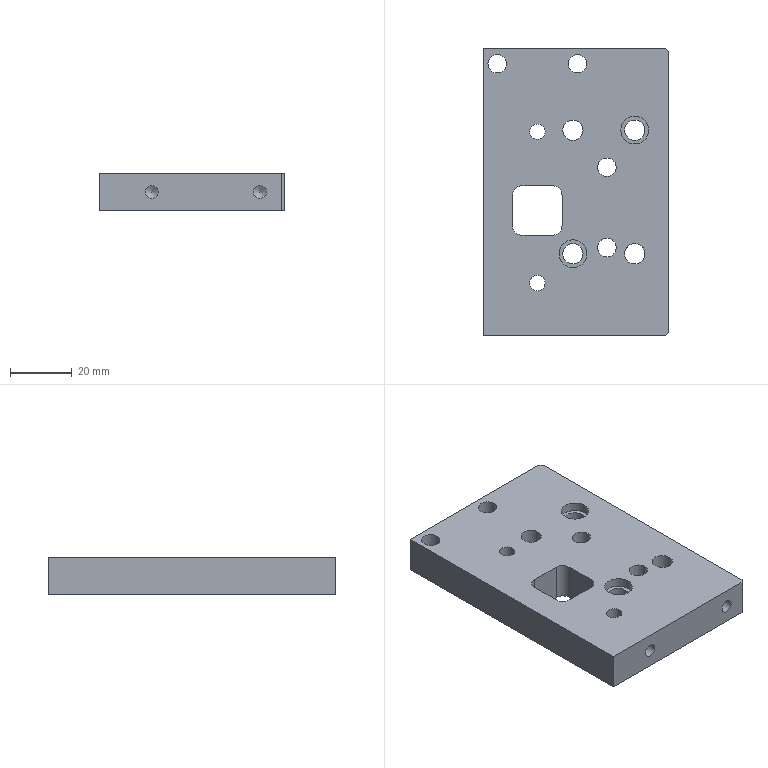Part | NX | features BREP 1 | 1 solid | 46 faces | box 60 x 93 x 12 mm | volume 58492 mm3 | cylinder 24 | plane 18 | cone 4 | commonest cylinder face diameters 6 x8 4.2 x4 6.6 x4 11 x4 5 x2 9 x2
STEP:
#1=CARTESIAN_POINT('',(29.,46.5,12.));
#2=VERTEX_POINT('',#1);
#3=CARTESIAN_POINT('',(-30.,46.5,12.));
#4=VERTEX_POINT('',#3);
#5=CARTESIAN_POINT('',(0.,46.5,12.));
#6=DIRECTION('',(-1.,0.,0.));
#7=VECTOR('',#6,1000.);
#8=LINE('',#5,#7);
#9=EDGE_CURVE('',#2,#4,#8,.T.);
#10=ORIENTED_EDGE('',*,*,#9,.T.);
#11=CARTESIAN_POINT('',(-30.,-46.5,12.));
#12=VERTEX_POINT('',#11);
#13=CARTESIAN_POINT('',(-30.,0.,12.));
#14=DIRECTION('',(0.,-1.,0.));
#15=VECTOR('',#14,1000.);
#16=LINE('',#13,#15);
#17=EDGE_CURVE('',#4,#12,#16,.T.);
#18=ORIENTED_EDGE('',*,*,#17,.T.);
#19=CARTESIAN_POINT('',(29.,-46.5,12.));
#20=VERTEX_POINT('',#19);
#21=CARTESIAN_POINT('',(0.,-46.5,12.));
#22=DIRECTION('',(1.,0.,0.));
#23=VECTOR('',#22,1000.);
#24=LINE('',#21,#23);
#25=EDGE_CURVE('',#12,#20,#24,.T.);
#26=ORIENTED_EDGE('',*,*,#25,.T.);
#27=CARTESIAN_POINT('',(30.,-45.5,12.));
#28=VERTEX_POINT('',#27);
#29=CARTESIAN_POINT('',(30.,-45.5,12.));
#30=DIRECTION('',(0.7071,0.7071,0.));
#31=VECTOR('',#30,1000.);
#32=LINE('',#29,#31);
#33=EDGE_CURVE('',#20,#28,#32,.T.);
#34=ORIENTED_EDGE('',*,*,#33,.T.);
#35=CARTESIAN_POINT('',(30.,45.5,12.));
#36=VERTEX_POINT('',#35);
#37=CARTESIAN_POINT('',(30.,0.,12.));
#38=DIRECTION('',(0.,1.,0.));
#39=VECTOR('',#38,1000.);
#40=LINE('',#37,#39);
#41=EDGE_CURVE('',#28,#36,#40,.T.);
#42=ORIENTED_EDGE('',*,*,#41,.T.);
#43=CARTESIAN_POINT('',(29.,46.5,12.));
#44=DIRECTION('',(-0.7071,0.7071,0.));
#45=VECTOR('',#44,1000.);
#46=LINE('',#43,#45);
#47=EDGE_CURVE('',#36,#2,#46,.T.);
#48=ORIENTED_EDGE('',*,*,#47,.T.);
#49=EDGE_LOOP('',(#10,#18,#26,#34,#42,#48));
#50=FACE_BOUND('',#49,.T.);
#51=CARTESIAN_POINT('',(-4.5,-1.,12.));
#52=VERTEX_POINT('',#51);
#53=CARTESIAN_POINT('',(-4.5,-11.,12.));
#54=VERTEX_POINT('',#53);
#55=CARTESIAN_POINT('',(-4.5,0.,12.));
#56=DIRECTION('',(0.,-1.,0.));
#57=VECTOR('',#56,1000.);
#58=LINE('',#55,#57);
#59=EDGE_CURVE('',#52,#54,#58,.T.);
#60=ORIENTED_EDGE('',*,*,#59,.T.);
#61=CARTESIAN_POINT('',(-7.5,-14.,12.));
#62=VERTEX_POINT('',#61);
#63=CARTESIAN_POINT('',(-7.5,-11.,12.));
#64=DIRECTION('',(0.,0.,-1.));
#65=DIRECTION('',(1.,0.,0.));
#66=AXIS2_PLACEMENT_3D('',#63,#64,#65);
#67=CIRCLE('',#66,3.);
#68=EDGE_CURVE('',#54,#62,#67,.T.);
#69=ORIENTED_EDGE('',*,*,#68,.T.);
#70=CARTESIAN_POINT('',(-17.5,-14.,12.));
#71=VERTEX_POINT('',#70);
#72=CARTESIAN_POINT('',(0.,-14.,12.));
#73=DIRECTION('',(-1.,0.,0.));
#74=VECTOR('',#73,1000.);
#75=LINE('',#72,#74);
#76=EDGE_CURVE('',#62,#71,#75,.T.);
#77=ORIENTED_EDGE('',*,*,#76,.T.);
#78=CARTESIAN_POINT('',(-20.5,-11.,12.));
#79=VERTEX_POINT('',#78);
#80=CARTESIAN_POINT('',(-17.5,-11.,12.));
#81=DIRECTION('',(0.,0.,-1.));
#82=DIRECTION('',(1.,0.,0.));
#83=AXIS2_PLACEMENT_3D('',#80,#81,#82);
#84=CIRCLE('',#83,3.);
#85=EDGE_CURVE('',#71,#79,#84,.T.);
#86=ORIENTED_EDGE('',*,*,#85,.T.);
#87=CARTESIAN_POINT('',(-20.5,-1.,12.));
#88=VERTEX_POINT('',#87);
#89=CARTESIAN_POINT('',(-20.5,0.,12.));
#90=DIRECTION('',(0.,1.,0.));
#91=VECTOR('',#90,1000.);
#92=LINE('',#89,#91);
#93=EDGE_CURVE('',#79,#88,#92,.T.);
#94=ORIENTED_EDGE('',*,*,#93,.T.);
#95=CARTESIAN_POINT('',(-17.5,2.,12.));
#96=VERTEX_POINT('',#95);
#97=CARTESIAN_POINT('',(-17.5,-1.,12.));
#98=DIRECTION('',(0.,0.,-1.));
#99=DIRECTION('',(1.,0.,0.));
#100=AXIS2_PLACEMENT_3D('',#97,#98,#99);
#101=CIRCLE('',#100,3.);
#102=EDGE_CURVE('',#88,#96,#101,.T.);
#103=ORIENTED_EDGE('',*,*,#102,.T.);
#104=CARTESIAN_POINT('',(-7.5,2.,12.));
#105=VERTEX_POINT('',#104);
#106=CARTESIAN_POINT('',(0.,2.,12.));
#107=DIRECTION('',(1.,0.,0.));
#108=VECTOR('',#107,1000.);
#109=LINE('',#106,#108);
#110=EDGE_CURVE('',#96,#105,#109,.T.);
#111=ORIENTED_EDGE('',*,*,#110,.T.);
#112=CARTESIAN_POINT('',(-7.5,-1.,12.));
#113=DIRECTION('',(0.,0.,-1.));
#114=DIRECTION('',(1.,0.,0.));
#115=AXIS2_PLACEMENT_3D('',#112,#113,#114);
#116=CIRCLE('',#115,3.);
#117=EDGE_CURVE('',#105,#52,#116,.T.);
#118=ORIENTED_EDGE('',*,*,#117,.T.);
#119=EDGE_LOOP('',(#60,#69,#77,#86,#94,#103,#111,#118));
#120=FACE_BOUND('',#119,.T.);
#121=CARTESIAN_POINT('',(-15.,-29.5,12.));
#122=VERTEX_POINT('',#121);
#123=CARTESIAN_POINT('',(-12.5,-29.5,12.));
#124=DIRECTION('',(0.,0.,-1.));
#125=DIRECTION('',(-1.,0.,0.));
#126=AXIS2_PLACEMENT_3D('',#123,#124,#125);
#127=CIRCLE('',#126,2.5);
#128=EDGE_CURVE('',#122,#122,#127,.T.);
#129=ORIENTED_EDGE('',*,*,#128,.T.);
#130=EDGE_LOOP('',(#129));
#131=FACE_BOUND('',#130,.T.);
#132=CARTESIAN_POINT('',(-15.,19.5,12.));
#133=VERTEX_POINT('',#132);
#134=CARTESIAN_POINT('',(-12.5,19.5,12.));
#135=DIRECTION('',(0.,0.,-1.));
#136=DIRECTION('',(-1.,0.,0.));
#137=AXIS2_PLACEMENT_3D('',#134,#135,#136);
#138=CIRCLE('',#137,2.5);
#139=EDGE_CURVE('',#133,#133,#138,.T.);
#140=ORIENTED_EDGE('',*,*,#139,.T.);
#141=EDGE_LOOP('',(#140));
#142=FACE_BOUND('',#141,.T.);
#143=CARTESIAN_POINT('',(15.7,-20.,12.));
#144=VERTEX_POINT('',#143);
#145=CARTESIAN_POINT('',(19.,-20.,12.));
#146=DIRECTION('',(0.,0.,-1.));
#147=DIRECTION('',(-1.,0.,0.));
#148=AXIS2_PLACEMENT_3D('',#145,#146,#147);
#149=CIRCLE('',#148,3.3);
#150=EDGE_CURVE('',#144,#144,#149,.T.);
#151=ORIENTED_EDGE('',*,*,#150,.T.);
#152=EDGE_LOOP('',(#151));
#153=FACE_BOUND('',#152,.T.);
#154=CARTESIAN_POINT('',(-4.3,20.,12.));
#155=VERTEX_POINT('',#154);
#156=CARTESIAN_POINT('',(-1.,20.,12.));
#157=DIRECTION('',(0.,0.,-1.));
#158=DIRECTION('',(-1.,0.,0.));
#159=AXIS2_PLACEMENT_3D('',#156,#157,#158);
#160=CIRCLE('',#159,3.3);
#161=EDGE_CURVE('',#155,#155,#160,.T.);
#162=ORIENTED_EDGE('',*,*,#161,.T.);
#163=EDGE_LOOP('',(#162));
#164=FACE_BOUND('',#163,.T.);
#165=CARTESIAN_POINT('',(7.,8.,12.));
#166=VERTEX_POINT('',#165);
#167=CARTESIAN_POINT('',(10.,8.,12.));
#168=DIRECTION('',(0.,0.,-1.));
#169=DIRECTION('',(-1.,0.,0.));
#170=AXIS2_PLACEMENT_3D('',#167,#168,#169);
#171=CIRCLE('',#170,3.);
#172=EDGE_CURVE('',#166,#166,#171,.T.);
#173=ORIENTED_EDGE('',*,*,#172,.T.);
#174=EDGE_LOOP('',(#173));
#175=FACE_BOUND('',#174,.T.);
#176=CARTESIAN_POINT('',(7.,-18.,12.));
#177=VERTEX_POINT('',#176);
#178=CARTESIAN_POINT('',(10.,-18.,12.));
#179=DIRECTION('',(0.,0.,-1.));
#180=DIRECTION('',(-1.,0.,0.));
#181=AXIS2_PLACEMENT_3D('',#178,#179,#180);
#182=CIRCLE('',#181,3.);
#183=EDGE_CURVE('',#177,#177,#182,.T.);
#184=ORIENTED_EDGE('',*,*,#183,.T.);
#185=EDGE_LOOP('',(#184));
#186=FACE_BOUND('',#185,.T.);
#187=CARTESIAN_POINT('',(-2.5,41.5,12.));
#188=VERTEX_POINT('',#187);
#189=CARTESIAN_POINT('',(0.5,41.5,12.));
#190=DIRECTION('',(0.,0.,-1.));
#191=DIRECTION('',(-1.,0.,0.));
#192=AXIS2_PLACEMENT_3D('',#189,#190,#191);
#193=CIRCLE('',#192,3.);
#194=EDGE_CURVE('',#188,#188,#193,.T.);
#195=ORIENTED_EDGE('',*,*,#194,.T.);
#196=EDGE_LOOP('',(#195));
#197=FACE_BOUND('',#196,.T.);
#198=CARTESIAN_POINT('',(-28.5,41.5,12.));
#199=VERTEX_POINT('',#198);
#200=CARTESIAN_POINT('',(-25.5,41.5,12.));
#201=DIRECTION('',(0.,0.,-1.));
#202=DIRECTION('',(-1.,0.,0.));
#203=AXIS2_PLACEMENT_3D('',#200,#201,#202);
#204=CIRCLE('',#203,3.);
#205=EDGE_CURVE('',#199,#199,#204,.T.);
#206=ORIENTED_EDGE('',*,*,#205,.T.);
#207=EDGE_LOOP('',(#206));
#208=FACE_BOUND('',#207,.T.);
#209=CARTESIAN_POINT('',(3.5,-20.,12.));
#210=VERTEX_POINT('',#209);
#211=CARTESIAN_POINT('',(-1.,-20.,12.));
#212=DIRECTION('',(0.,0.,-1.));
#213=DIRECTION('',(1.,0.,0.));
#214=AXIS2_PLACEMENT_3D('',#211,#212,#213);
#215=CIRCLE('',#214,4.5);
#216=EDGE_CURVE('',#210,#210,#215,.T.);
#217=ORIENTED_EDGE('',*,*,#216,.T.);
#218=EDGE_LOOP('',(#217));
#219=FACE_BOUND('',#218,.T.);
#220=CARTESIAN_POINT('',(23.5,20.,12.));
#221=VERTEX_POINT('',#220);
#222=CARTESIAN_POINT('',(19.,20.,12.));
#223=DIRECTION('',(0.,0.,-1.));
#224=DIRECTION('',(1.,0.,0.));
#225=AXIS2_PLACEMENT_3D('',#222,#223,#224);
#226=CIRCLE('',#225,4.5);
#227=EDGE_CURVE('',#221,#221,#226,.T.);
#228=ORIENTED_EDGE('',*,*,#227,.T.);
#229=EDGE_LOOP('',(#228));
#230=FACE_BOUND('',#229,.T.);
#231=CARTESIAN_POINT('',(0.,0.,12.));
#232=DIRECTION('',(0.,0.,1.));
#233=DIRECTION('',(-1.,0.,0.));
#234=AXIS2_PLACEMENT_3D('',#231,#232,#233);
#235=PLANE('',#234);
#236=ADVANCED_FACE('',(#50,#120,#131,#142,#153,#164,#175,#186,#197,#208,#219,#230),#235,.T.);
#237=CARTESIAN_POINT('',(-30.,-46.5,0.));
#238=VERTEX_POINT('',#237);
#239=CARTESIAN_POINT('',(-30.,-46.5,12.));
#240=DIRECTION('',(0.,0.,-1.));
#241=VECTOR('',#240,1000.);
#242=LINE('',#239,#241);
#243=EDGE_CURVE('',#12,#238,#242,.T.);
#244=ORIENTED_EDGE('',*,*,#243,.F.);
#245=ORIENTED_EDGE('',*,*,#17,.F.);
#246=CARTESIAN_POINT('',(-30.,46.5,0.));
#247=VERTEX_POINT('',#246);
#248=CARTESIAN_POINT('',(-30.,46.5,12.));
#249=DIRECTION('',(0.,0.,1.));
#250=VECTOR('',#249,1000.);
#251=LINE('',#248,#250);
#252=EDGE_CURVE('',#247,#4,#251,.T.);
#253=ORIENTED_EDGE('',*,*,#252,.F.);
#254=CARTESIAN_POINT('',(-30.,46.5,0.));
#255=DIRECTION('',(0.,1.,0.));
#256=VECTOR('',#255,1000.);
#257=LINE('',#254,#256);
#258=EDGE_CURVE('',#238,#247,#257,.T.);
#259=ORIENTED_EDGE('',*,*,#258,.F.);
#260=EDGE_LOOP('',(#244,#245,#253,#259));
#261=FACE_BOUND('',#260,.T.);
#262=CARTESIAN_POINT('',(-30.,46.5,12.));
#263=DIRECTION('',(1.,0.,0.));
#264=DIRECTION('',(0.,-1.,0.));
#265=AXIS2_PLACEMENT_3D('',#262,#263,#264);
#266=PLANE('',#265);
#267=ADVANCED_FACE('',(#261),#266,.F.);
#268=CARTESIAN_POINT('',(29.,46.5,0.));
#269=VERTEX_POINT('',#268);
#270=CARTESIAN_POINT('',(29.,46.5,12.));
#271=DIRECTION('',(0.,0.,1.));
#272=VECTOR('',#271,1000.);
#273=LINE('',#270,#272);
#274=EDGE_CURVE('',#269,#2,#273,.T.);
#275=ORIENTED_EDGE('',*,*,#274,.F.);
#276=CARTESIAN_POINT('',(-30.,46.5,0.));
#277=DIRECTION('',(1.,0.,0.));
#278=VECTOR('',#277,1000.);
#279=LINE('',#276,#278);
#280=EDGE_CURVE('',#247,#269,#279,.T.);
#281=ORIENTED_EDGE('',*,*,#280,.F.);
#282=ORIENTED_EDGE('',*,*,#252,.T.);
#283=ORIENTED_EDGE('',*,*,#9,.F.);
#284=EDGE_LOOP('',(#275,#281,#282,#283));
#285=FACE_BOUND('',#284,.T.);
#286=CARTESIAN_POINT('',(-13.,46.5,8.1));
#287=VERTEX_POINT('',#286);
#288=CARTESIAN_POINT('',(-13.,46.5,6.));
#289=DIRECTION('',(0.,1.,0.));
#290=DIRECTION('',(0.,0.,1.));
#291=AXIS2_PLACEMENT_3D('',#288,#289,#290);
#292=CIRCLE('',#291,2.1);
#293=EDGE_CURVE('',#287,#287,#292,.T.);
#294=ORIENTED_EDGE('',*,*,#293,.F.);
#295=EDGE_LOOP('',(#294));
#296=FACE_BOUND('',#295,.T.);
#297=CARTESIAN_POINT('',(22.,46.5,8.1));
#298=VERTEX_POINT('',#297);
#299=CARTESIAN_POINT('',(22.,46.5,6.));
#300=DIRECTION('',(0.,1.,0.));
#301=DIRECTION('',(0.,0.,1.));
#302=AXIS2_PLACEMENT_3D('',#299,#300,#301);
#303=CIRCLE('',#302,2.1);
#304=EDGE_CURVE('',#298,#298,#303,.T.);
#305=ORIENTED_EDGE('',*,*,#304,.F.);
#306=EDGE_LOOP('',(#305));
#307=FACE_BOUND('',#306,.T.);
#308=CARTESIAN_POINT('',(-30.,46.5,12.));
#309=DIRECTION('',(0.,-1.,0.));
#310=DIRECTION('',(0.,0.,1.));
#311=AXIS2_PLACEMENT_3D('',#308,#309,#310);
#312=PLANE('',#311);
#313=ADVANCED_FACE('',(#285,#296,#307),#312,.F.);
#314=CARTESIAN_POINT('',(30.,-45.5,0.));
#315=VERTEX_POINT('',#314);
#316=CARTESIAN_POINT('',(30.,-45.5,12.));
#317=DIRECTION('',(0.,0.,1.));
#318=VECTOR('',#317,1000.);
#319=LINE('',#316,#318);
#320=EDGE_CURVE('',#315,#28,#319,.T.);
#321=ORIENTED_EDGE('',*,*,#320,.F.);
#322=CARTESIAN_POINT('',(30.,45.5,0.));
#323=VERTEX_POINT('',#322);
#324=CARTESIAN_POINT('',(30.,46.5,0.));
#325=DIRECTION('',(0.,-1.,0.));
#326=VECTOR('',#325,1000.);
#327=LINE('',#324,#326);
#328=EDGE_CURVE('',#323,#315,#327,.T.);
#329=ORIENTED_EDGE('',*,*,#328,.F.);
#330=CARTESIAN_POINT('',(30.,45.5,12.));
#331=DIRECTION('',(0.,0.,-1.));
#332=VECTOR('',#331,1000.);
#333=LINE('',#330,#332);
#334=EDGE_CURVE('',#36,#323,#333,.T.);
#335=ORIENTED_EDGE('',*,*,#334,.F.);
#336=ORIENTED_EDGE('',*,*,#41,.F.);
#337=EDGE_LOOP('',(#321,#329,#335,#336));
#338=FACE_BOUND('',#337,.T.);
#339=CARTESIAN_POINT('',(30.,46.5,12.));
#340=DIRECTION('',(-1.,0.,0.));
#341=DIRECTION('',(0.,1.,0.));
#342=AXIS2_PLACEMENT_3D('',#339,#340,#341);
#343=PLANE('',#342);
#344=ADVANCED_FACE('',(#338),#343,.F.);
#345=CARTESIAN_POINT('',(29.,-46.5,0.));
#346=VERTEX_POINT('',#345);
#347=CARTESIAN_POINT('',(29.,-46.5,12.));
#348=DIRECTION('',(0.,0.,-1.));
#349=VECTOR('',#348,1000.);
#350=LINE('',#347,#349);
#351=EDGE_CURVE('',#20,#346,#350,.T.);
#352=ORIENTED_EDGE('',*,*,#351,.F.);
#353=ORIENTED_EDGE('',*,*,#25,.F.);
#354=ORIENTED_EDGE('',*,*,#243,.T.);
#355=CARTESIAN_POINT('',(-30.,-46.5,0.));
#356=DIRECTION('',(-1.,0.,0.));
#357=VECTOR('',#356,1000.);
#358=LINE('',#355,#357);
#359=EDGE_CURVE('',#346,#238,#358,.T.);
#360=ORIENTED_EDGE('',*,*,#359,.F.);
#361=EDGE_LOOP('',(#352,#353,#354,#360));
#362=FACE_BOUND('',#361,.T.);
#363=CARTESIAN_POINT('',(-13.,-46.5,3.9));
#364=VERTEX_POINT('',#363);
#365=CARTESIAN_POINT('',(-13.,-46.5,6.));
#366=DIRECTION('',(0.,-1.,0.));
#367=DIRECTION('',(0.,0.,-1.));
#368=AXIS2_PLACEMENT_3D('',#365,#366,#367);
#369=CIRCLE('',#368,2.1);
#370=EDGE_CURVE('',#364,#364,#369,.T.);
#371=ORIENTED_EDGE('',*,*,#370,.F.);
#372=EDGE_LOOP('',(#371));
#373=FACE_BOUND('',#372,.T.);
#374=CARTESIAN_POINT('',(22.,-46.5,3.9));
#375=VERTEX_POINT('',#374);
#376=CARTESIAN_POINT('',(22.,-46.5,6.));
#377=DIRECTION('',(0.,-1.,0.));
#378=DIRECTION('',(0.,0.,-1.));
#379=AXIS2_PLACEMENT_3D('',#376,#377,#378);
#380=CIRCLE('',#379,2.1);
#381=EDGE_CURVE('',#375,#375,#380,.T.);
#382=ORIENTED_EDGE('',*,*,#381,.F.);
#383=EDGE_LOOP('',(#382));
#384=FACE_BOUND('',#383,.T.);
#385=CARTESIAN_POINT('',(-30.,-46.5,12.));
#386=DIRECTION('',(0.,1.,0.));
#387=DIRECTION('',(0.,0.,-1.));
#388=AXIS2_PLACEMENT_3D('',#385,#386,#387);
#389=PLANE('',#388);
#390=ADVANCED_FACE('',(#362,#373,#384),#389,.F.);
#391=CARTESIAN_POINT('',(-4.5,-11.,0.));
#392=VERTEX_POINT('',#391);
#393=CARTESIAN_POINT('',(-4.5,-11.,12.));
#394=DIRECTION('',(0.,0.,1.));
#395=VECTOR('',#394,1000.);
#396=LINE('',#393,#395);
#397=EDGE_CURVE('',#392,#54,#396,.T.);
#398=ORIENTED_EDGE('',*,*,#397,.F.);
#399=CARTESIAN_POINT('',(-7.5,-14.,0.));
#400=VERTEX_POINT('',#399);
#401=CARTESIAN_POINT('',(-7.5,-11.,0.));
#402=DIRECTION('',(0.,0.,1.));
#403=DIRECTION('',(1.,0.,0.));
#404=AXIS2_PLACEMENT_3D('',#401,#402,#403);
#405=CIRCLE('',#404,3.);
#406=EDGE_CURVE('',#400,#392,#405,.T.);
#407=ORIENTED_EDGE('',*,*,#406,.F.);
#408=CARTESIAN_POINT('',(-7.5,-14.,12.));
#409=DIRECTION('',(0.,0.,-1.));
#410=VECTOR('',#409,1000.);
#411=LINE('',#408,#410);
#412=EDGE_CURVE('',#62,#400,#411,.T.);
#413=ORIENTED_EDGE('',*,*,#412,.F.);
#414=ORIENTED_EDGE('',*,*,#68,.F.);
#415=EDGE_LOOP('',(#398,#407,#413,#414));
#416=FACE_BOUND('',#415,.T.);
#417=CARTESIAN_POINT('',(-7.5,-11.,12.));
#418=DIRECTION('',(0.,0.,1.));
#419=DIRECTION('',(-1.,0.,0.));
#420=AXIS2_PLACEMENT_3D('',#417,#418,#419);
#421=CYLINDRICAL_SURFACE('',#420,3.);
#422=ADVANCED_FACE('',(#416),#421,.F.);
#423=ORIENTED_EDGE('',*,*,#397,.T.);
#424=ORIENTED_EDGE('',*,*,#59,.F.);
#425=CARTESIAN_POINT('',(-4.5,-1.,0.));
#426=VERTEX_POINT('',#425);
#427=CARTESIAN_POINT('',(-4.5,-1.,12.));
#428=DIRECTION('',(0.,0.,1.));
#429=VECTOR('',#428,1000.);
#430=LINE('',#427,#429);
#431=EDGE_CURVE('',#426,#52,#430,.T.);
#432=ORIENTED_EDGE('',*,*,#431,.F.);
#433=CARTESIAN_POINT('',(-4.5,2.,0.));
#434=DIRECTION('',(0.,1.,0.));
#435=VECTOR('',#434,1000.);
#436=LINE('',#433,#435);
#437=EDGE_CURVE('',#392,#426,#436,.T.);
#438=ORIENTED_EDGE('',*,*,#437,.F.);
#439=EDGE_LOOP('',(#423,#424,#432,#438));
#440=FACE_BOUND('',#439,.T.);
#441=CARTESIAN_POINT('',(-4.5,2.,12.));
#442=DIRECTION('',(1.,0.,0.));
#443=DIRECTION('',(0.,-1.,0.));
#444=AXIS2_PLACEMENT_3D('',#441,#442,#443);
#445=PLANE('',#444);
#446=ADVANCED_FACE('',(#440),#445,.F.);
#447=CARTESIAN_POINT('',(-7.5,2.,0.));
#448=VERTEX_POINT('',#447);
#449=CARTESIAN_POINT('',(-7.5,2.,12.));
#450=DIRECTION('',(0.,0.,1.));
#451=VECTOR('',#450,1000.);
#452=LINE('',#449,#451);
#453=EDGE_CURVE('',#448,#105,#452,.T.);
#454=ORIENTED_EDGE('',*,*,#453,.F.);
#455=CARTESIAN_POINT('',(-7.5,-1.,0.));
#456=DIRECTION('',(0.,0.,1.));
#457=DIRECTION('',(1.,0.,0.));
#458=AXIS2_PLACEMENT_3D('',#455,#456,#457);
#459=CIRCLE('',#458,3.);
#460=EDGE_CURVE('',#426,#448,#459,.T.);
#461=ORIENTED_EDGE('',*,*,#460,.F.);
#462=ORIENTED_EDGE('',*,*,#431,.T.);
#463=ORIENTED_EDGE('',*,*,#117,.F.);
#464=EDGE_LOOP('',(#454,#461,#462,#463));
#465=FACE_BOUND('',#464,.T.);
#466=CARTESIAN_POINT('',(-7.5,-1.,12.));
#467=DIRECTION('',(0.,0.,1.));
#468=DIRECTION('',(-1.,0.,0.));
#469=AXIS2_PLACEMENT_3D('',#466,#467,#468);
#470=CYLINDRICAL_SURFACE('',#469,3.);
#471=ADVANCED_FACE('',(#465),#470,.F.);
#472=CARTESIAN_POINT('',(-17.5,2.,0.));
#473=VERTEX_POINT('',#472);
#474=CARTESIAN_POINT('',(-17.5,2.,12.));
#475=DIRECTION('',(0.,0.,1.));
#476=VECTOR('',#475,1000.);
#477=LINE('',#474,#476);
#478=EDGE_CURVE('',#473,#96,#477,.T.);
#479=ORIENTED_EDGE('',*,*,#478,.F.);
#480=CARTESIAN_POINT('',(-4.5,2.,0.));
#481=DIRECTION('',(-1.,0.,0.));
#482=VECTOR('',#481,1000.);
#483=LINE('',#480,#482);
#484=EDGE_CURVE('',#448,#473,#483,.T.);
#485=ORIENTED_EDGE('',*,*,#484,.F.);
#486=ORIENTED_EDGE('',*,*,#453,.T.);
#487=ORIENTED_EDGE('',*,*,#110,.F.);
#488=EDGE_LOOP('',(#479,#485,#486,#487));
#489=FACE_BOUND('',#488,.T.);
#490=CARTESIAN_POINT('',(-4.5,2.,12.));
#491=DIRECTION('',(0.,1.,0.));
#492=DIRECTION('',(0.,0.,-1.));
#493=AXIS2_PLACEMENT_3D('',#490,#491,#492);
#494=PLANE('',#493);
#495=ADVANCED_FACE('',(#489),#494,.F.);
#496=CARTESIAN_POINT('',(-20.5,-1.,0.));
#497=VERTEX_POINT('',#496);
#498=CARTESIAN_POINT('',(-20.5,-1.,12.));
#499=DIRECTION('',(0.,0.,1.));
#500=VECTOR('',#499,1000.);
#501=LINE('',#498,#500);
#502=EDGE_CURVE('',#497,#88,#501,.T.);
#503=ORIENTED_EDGE('',*,*,#502,.F.);
#504=CARTESIAN_POINT('',(-17.5,-1.,0.));
#505=DIRECTION('',(0.,0.,1.));
#506=DIRECTION('',(1.,0.,0.));
#507=AXIS2_PLACEMENT_3D('',#504,#505,#506);
#508=CIRCLE('',#507,3.);
#509=EDGE_CURVE('',#473,#497,#508,.T.);
#510=ORIENTED_EDGE('',*,*,#509,.F.);
#511=ORIENTED_EDGE('',*,*,#478,.T.);
#512=ORIENTED_EDGE('',*,*,#102,.F.);
#513=EDGE_LOOP('',(#503,#510,#511,#512));
#514=FACE_BOUND('',#513,.T.);
#515=CARTESIAN_POINT('',(-17.5,-1.,12.));
#516=DIRECTION('',(0.,0.,1.));
#517=DIRECTION('',(-1.,0.,0.));
#518=AXIS2_PLACEMENT_3D('',#515,#516,#517);
#519=CYLINDRICAL_SURFACE('',#518,3.);
#520=ADVANCED_FACE('',(#514),#519,.F.);
#521=CARTESIAN_POINT('',(-20.5,-11.,0.));
#522=VERTEX_POINT('',#521);
#523=CARTESIAN_POINT('',(-20.5,-11.,12.));
#524=DIRECTION('',(0.,0.,1.));
#525=VECTOR('',#524,1000.);
#526=LINE('',#523,#525);
#527=EDGE_CURVE('',#522,#79,#526,.T.);
#528=ORIENTED_EDGE('',*,*,#527,.F.);
#529=CARTESIAN_POINT('',(-20.5,2.,0.));
#530=DIRECTION('',(0.,-1.,0.));
#531=VECTOR('',#530,1000.);
#532=LINE('',#529,#531);
#533=EDGE_CURVE('',#497,#522,#532,.T.);
#534=ORIENTED_EDGE('',*,*,#533,.F.);
#535=ORIENTED_EDGE('',*,*,#502,.T.);
#536=ORIENTED_EDGE('',*,*,#93,.F.);
#537=EDGE_LOOP('',(#528,#534,#535,#536));
#538=FACE_BOUND('',#537,.T.);
#539=CARTESIAN_POINT('',(-20.5,2.,12.));
#540=DIRECTION('',(-1.,0.,0.));
#541=DIRECTION('',(0.,0.,-1.));
#542=AXIS2_PLACEMENT_3D('',#539,#540,#541);
#543=PLANE('',#542);
#544=ADVANCED_FACE('',(#538),#543,.F.);
#545=CARTESIAN_POINT('',(-17.5,-14.,0.));
#546=VERTEX_POINT('',#545);
#547=CARTESIAN_POINT('',(-17.5,-14.,12.));
#548=DIRECTION('',(0.,0.,1.));
#549=VECTOR('',#548,1000.);
#550=LINE('',#547,#549);
#551=EDGE_CURVE('',#546,#71,#550,.T.);
#552=ORIENTED_EDGE('',*,*,#551,.F.);
#553=CARTESIAN_POINT('',(-17.5,-11.,0.));
#554=DIRECTION('',(0.,0.,1.));
#555=DIRECTION('',(1.,0.,0.));
#556=AXIS2_PLACEMENT_3D('',#553,#554,#555);
#557=CIRCLE('',#556,3.);
#558=EDGE_CURVE('',#522,#546,#557,.T.);
#559=ORIENTED_EDGE('',*,*,#558,.F.);
#560=ORIENTED_EDGE('',*,*,#527,.T.);
#561=ORIENTED_EDGE('',*,*,#85,.F.);
#562=EDGE_LOOP('',(#552,#559,#560,#561));
#563=FACE_BOUND('',#562,.T.);
#564=CARTESIAN_POINT('',(-17.5,-11.,12.));
#565=DIRECTION('',(0.,0.,1.));
#566=DIRECTION('',(-1.,0.,0.));
#567=AXIS2_PLACEMENT_3D('',#564,#565,#566);
#568=CYLINDRICAL_SURFACE('',#567,3.);
#569=ADVANCED_FACE('',(#563),#568,.F.);
#570=ORIENTED_EDGE('',*,*,#412,.T.);
#571=CARTESIAN_POINT('',(-4.5,-14.,0.));
#572=DIRECTION('',(1.,0.,0.));
#573=VECTOR('',#572,1000.);
#574=LINE('',#571,#573);
#575=EDGE_CURVE('',#546,#400,#574,.T.);
#576=ORIENTED_EDGE('',*,*,#575,.F.);
#577=ORIENTED_EDGE('',*,*,#551,.T.);
#578=ORIENTED_EDGE('',*,*,#76,.F.);
#579=EDGE_LOOP('',(#570,#576,#577,#578));
#580=FACE_BOUND('',#579,.T.);
#581=CARTESIAN_POINT('',(-4.5,-14.,12.));
#582=DIRECTION('',(0.,-1.,0.));
#583=DIRECTION('',(0.,0.,1.));
#584=AXIS2_PLACEMENT_3D('',#581,#582,#583);
#585=PLANE('',#584);
#586=ADVANCED_FACE('',(#580),#585,.F.);
#587=CARTESIAN_POINT('',(-15.,-29.5,0.));
#588=VERTEX_POINT('',#587);
#589=CARTESIAN_POINT('',(-12.5,-29.5,0.));
#590=DIRECTION('',(0.,0.,1.));
#591=DIRECTION('',(-1.,0.,0.));
#592=AXIS2_PLACEMENT_3D('',#589,#590,#591);
#593=CIRCLE('',#592,2.5);
#594=EDGE_CURVE('',#588,#588,#593,.T.);
#595=ORIENTED_EDGE('',*,*,#594,.F.);
#596=EDGE_LOOP('',(#595));
#597=FACE_BOUND('',#596,.T.);
#598=ORIENTED_EDGE('',*,*,#128,.F.);
#599=EDGE_LOOP('',(#598));
#600=FACE_BOUND('',#599,.T.);
#601=CARTESIAN_POINT('',(-12.5,-29.5,0.));
#602=DIRECTION('',(0.,0.,-1.));
#603=DIRECTION('',(1.,0.,0.));
#604=AXIS2_PLACEMENT_3D('',#601,#602,#603);
#605=CYLINDRICAL_SURFACE('',#604,2.5);
#606=ADVANCED_FACE('',(#597,#600),#605,.F.);
#607=CARTESIAN_POINT('',(-15.,19.5,0.));
#608=VERTEX_POINT('',#607);
#609=CARTESIAN_POINT('',(-12.5,19.5,0.));
#610=DIRECTION('',(0.,0.,1.));
#611=DIRECTION('',(-1.,0.,0.));
#612=AXIS2_PLACEMENT_3D('',#609,#610,#611);
#613=CIRCLE('',#612,2.5);
#614=EDGE_CURVE('',#608,#608,#613,.T.);
#615=ORIENTED_EDGE('',*,*,#614,.F.);
#616=EDGE_LOOP('',(#615));
#617=FACE_BOUND('',#616,.T.);
#618=ORIENTED_EDGE('',*,*,#139,.F.);
#619=EDGE_LOOP('',(#618));
#620=FACE_BOUND('',#619,.T.);
#621=CARTESIAN_POINT('',(-12.5,19.5,0.));
#622=DIRECTION('',(0.,0.,-1.));
#623=DIRECTION('',(1.,0.,0.));
#624=AXIS2_PLACEMENT_3D('',#621,#622,#623);
#625=CYLINDRICAL_SURFACE('',#624,2.5);
#626=ADVANCED_FACE('',(#617,#620),#625,.F.);
#627=CARTESIAN_POINT('',(15.7,-20.,4.6));
#628=VERTEX_POINT('',#627);
#629=CARTESIAN_POINT('',(19.,-20.,4.6));
#630=DIRECTION('',(0.,0.,1.));
#631=DIRECTION('',(-1.,0.,0.));
#632=AXIS2_PLACEMENT_3D('',#629,#630,#631);
#633=CIRCLE('',#632,3.3);
#634=EDGE_CURVE('',#628,#628,#633,.T.);
#635=ORIENTED_EDGE('',*,*,#634,.F.);
#636=EDGE_LOOP('',(#635));
#637=FACE_BOUND('',#636,.T.);
#638=ORIENTED_EDGE('',*,*,#150,.F.);
#639=EDGE_LOOP('',(#638));
#640=FACE_BOUND('',#639,.T.);
#641=CARTESIAN_POINT('',(19.,-20.,0.));
#642=DIRECTION('',(0.,0.,-1.));
#643=DIRECTION('',(1.,0.,0.));
#644=AXIS2_PLACEMENT_3D('',#641,#642,#643);
#645=CYLINDRICAL_SURFACE('',#644,3.3);
#646=ADVANCED_FACE('',(#637,#640),#645,.F.);
#647=CARTESIAN_POINT('',(-4.3,20.,4.6));
#648=VERTEX_POINT('',#647);
#649=CARTESIAN_POINT('',(-1.,20.,4.6));
#650=DIRECTION('',(0.,0.,1.));
#651=DIRECTION('',(-1.,0.,0.));
#652=AXIS2_PLACEMENT_3D('',#649,#650,#651);
#653=CIRCLE('',#652,3.3);
#654=EDGE_CURVE('',#648,#648,#653,.T.);
#655=ORIENTED_EDGE('',*,*,#654,.F.);
#656=EDGE_LOOP('',(#655));
#657=FACE_BOUND('',#656,.T.);
#658=ORIENTED_EDGE('',*,*,#161,.F.);
#659=EDGE_LOOP('',(#658));
#660=FACE_BOUND('',#659,.T.);
#661=CARTESIAN_POINT('',(-1.,20.,0.));
#662=DIRECTION('',(0.,0.,-1.));
#663=DIRECTION('',(1.,0.,0.));
#664=AXIS2_PLACEMENT_3D('',#661,#662,#663);
#665=CYLINDRICAL_SURFACE('',#664,3.3);
#666=ADVANCED_FACE('',(#657,#660),#665,.F.);
#667=CARTESIAN_POINT('',(7.,8.,0.));
#668=VERTEX_POINT('',#667);
#669=CARTESIAN_POINT('',(10.,8.,0.));
#670=DIRECTION('',(0.,0.,1.));
#671=DIRECTION('',(-1.,0.,0.));
#672=AXIS2_PLACEMENT_3D('',#669,#670,#671);
#673=CIRCLE('',#672,3.);
#674=EDGE_CURVE('',#668,#668,#673,.T.);
#675=ORIENTED_EDGE('',*,*,#674,.F.);
#676=EDGE_LOOP('',(#675));
#677=FACE_BOUND('',#676,.T.);
#678=ORIENTED_EDGE('',*,*,#172,.F.);
#679=EDGE_LOOP('',(#678));
#680=FACE_BOUND('',#679,.T.);
#681=CARTESIAN_POINT('',(10.,8.,0.));
#682=DIRECTION('',(0.,0.,-1.));
#683=DIRECTION('',(1.,0.,0.));
#684=AXIS2_PLACEMENT_3D('',#681,#682,#683);
#685=CYLINDRICAL_SURFACE('',#684,3.);
#686=ADVANCED_FACE('',(#677,#680),#685,.F.);
#687=CARTESIAN_POINT('',(7.,-18.,0.));
#688=VERTEX_POINT('',#687);
#689=CARTESIAN_POINT('',(10.,-18.,0.));
#690=DIRECTION('',(0.,0.,1.));
#691=DIRECTION('',(-1.,0.,0.));
#692=AXIS2_PLACEMENT_3D('',#689,#690,#691);
#693=CIRCLE('',#692,3.);
#694=EDGE_CURVE('',#688,#688,#693,.T.);
#695=ORIENTED_EDGE('',*,*,#694,.F.);
#696=EDGE_LOOP('',(#695));
#697=FACE_BOUND('',#696,.T.);
#698=ORIENTED_EDGE('',*,*,#183,.F.);
#699=EDGE_LOOP('',(#698));
#700=FACE_BOUND('',#699,.T.);
#701=CARTESIAN_POINT('',(10.,-18.,0.));
#702=DIRECTION('',(0.,0.,-1.));
#703=DIRECTION('',(1.,0.,0.));
#704=AXIS2_PLACEMENT_3D('',#701,#702,#703);
#705=CYLINDRICAL_SURFACE('',#704,3.);
#706=ADVANCED_FACE('',(#697,#700),#705,.F.);
#707=CARTESIAN_POINT('',(-2.5,41.5,0.));
#708=VERTEX_POINT('',#707);
#709=CARTESIAN_POINT('',(0.5,41.5,0.));
#710=DIRECTION('',(0.,0.,1.));
#711=DIRECTION('',(-1.,0.,0.));
#712=AXIS2_PLACEMENT_3D('',#709,#710,#711);
#713=CIRCLE('',#712,3.);
#714=EDGE_CURVE('',#708,#708,#713,.T.);
#715=ORIENTED_EDGE('',*,*,#714,.F.);
#716=EDGE_LOOP('',(#715));
#717=FACE_BOUND('',#716,.T.);
#718=ORIENTED_EDGE('',*,*,#194,.F.);
#719=EDGE_LOOP('',(#718));
#720=FACE_BOUND('',#719,.T.);
#721=CARTESIAN_POINT('',(0.5,41.5,0.));
#722=DIRECTION('',(0.,0.,-1.));
#723=DIRECTION('',(1.,0.,0.));
#724=AXIS2_PLACEMENT_3D('',#721,#722,#723);
#725=CYLINDRICAL_SURFACE('',#724,3.);
#726=ADVANCED_FACE('',(#717,#720),#725,.F.);
#727=CARTESIAN_POINT('',(-28.5,41.5,0.));
#728=VERTEX_POINT('',#727);
#729=CARTESIAN_POINT('',(-25.5,41.5,0.));
#730=DIRECTION('',(0.,0.,1.));
#731=DIRECTION('',(-1.,0.,0.));
#732=AXIS2_PLACEMENT_3D('',#729,#730,#731);
#733=CIRCLE('',#732,3.);
#734=EDGE_CURVE('',#728,#728,#733,.T.);
#735=ORIENTED_EDGE('',*,*,#734,.F.);
#736=EDGE_LOOP('',(#735));
#737=FACE_BOUND('',#736,.T.);
#738=ORIENTED_EDGE('',*,*,#205,.F.);
#739=EDGE_LOOP('',(#738));
#740=FACE_BOUND('',#739,.T.);
#741=CARTESIAN_POINT('',(-25.5,41.5,0.));
#742=DIRECTION('',(0.,0.,-1.));
#743=DIRECTION('',(1.,0.,0.));
#744=AXIS2_PLACEMENT_3D('',#741,#742,#743);
#745=CYLINDRICAL_SURFACE('',#744,3.);
#746=ADVANCED_FACE('',(#737,#740),#745,.F.);
#747=ORIENTED_EDGE('',*,*,#216,.F.);
#748=EDGE_LOOP('',(#747));
#749=FACE_BOUND('',#748,.T.);
#750=CARTESIAN_POINT('',(3.5,-20.,9.));
#751=VERTEX_POINT('',#750);
#752=CARTESIAN_POINT('',(-1.,-20.,9.));
#753=DIRECTION('',(0.,0.,1.));
#754=DIRECTION('',(1.,0.,0.));
#755=AXIS2_PLACEMENT_3D('',#752,#753,#754);
#756=CIRCLE('',#755,4.5);
#757=EDGE_CURVE('',#751,#751,#756,.T.);
#758=ORIENTED_EDGE('',*,*,#757,.F.);
#759=EDGE_LOOP('',(#758));
#760=FACE_BOUND('',#759,.T.);
#761=CARTESIAN_POINT('',(-1.,-20.,9.));
#762=DIRECTION('',(0.,0.,1.));
#763=DIRECTION('',(-1.,0.,0.));
#764=AXIS2_PLACEMENT_3D('',#761,#762,#763);
#765=CYLINDRICAL_SURFACE('',#764,4.5);
#766=ADVANCED_FACE('',(#749,#760),#765,.F.);
#767=ORIENTED_EDGE('',*,*,#227,.F.);
#768=EDGE_LOOP('',(#767));
#769=FACE_BOUND('',#768,.T.);
#770=CARTESIAN_POINT('',(23.5,20.,9.));
#771=VERTEX_POINT('',#770);
#772=CARTESIAN_POINT('',(19.,20.,9.));
#773=DIRECTION('',(0.,0.,1.));
#774=DIRECTION('',(1.,0.,0.));
#775=AXIS2_PLACEMENT_3D('',#772,#773,#774);
#776=CIRCLE('',#775,4.5);
#777=EDGE_CURVE('',#771,#771,#776,.T.);
#778=ORIENTED_EDGE('',*,*,#777,.F.);
#779=EDGE_LOOP('',(#778));
#780=FACE_BOUND('',#779,.T.);
#781=CARTESIAN_POINT('',(19.,20.,9.));
#782=DIRECTION('',(0.,0.,1.));
#783=DIRECTION('',(-1.,0.,0.));
#784=AXIS2_PLACEMENT_3D('',#781,#782,#783);
#785=CYLINDRICAL_SURFACE('',#784,4.5);
#786=ADVANCED_FACE('',(#769,#780),#785,.F.);
#787=CARTESIAN_POINT('',(29.,-46.5,0.));
#788=DIRECTION('',(0.7071,0.7071,0.));
#789=VECTOR('',#788,1000.);
#790=LINE('',#787,#789);
#791=EDGE_CURVE('',#346,#315,#790,.T.);
#792=ORIENTED_EDGE('',*,*,#791,.F.);
#793=ORIENTED_EDGE('',*,*,#359,.T.);
#794=ORIENTED_EDGE('',*,*,#258,.T.);
#795=ORIENTED_EDGE('',*,*,#280,.T.);
#796=CARTESIAN_POINT('',(30.,45.5,0.));
#797=DIRECTION('',(-0.7071,0.7071,0.));
#798=VECTOR('',#797,1000.);
#799=LINE('',#796,#798);
#800=EDGE_CURVE('',#323,#269,#799,.T.);
#801=ORIENTED_EDGE('',*,*,#800,.F.);
#802=ORIENTED_EDGE('',*,*,#328,.T.);
#803=EDGE_LOOP('',(#792,#793,#794,#795,#801,#802));
#804=FACE_BOUND('',#803,.T.);
#805=ORIENTED_EDGE('',*,*,#509,.T.);
#806=ORIENTED_EDGE('',*,*,#533,.T.);
#807=ORIENTED_EDGE('',*,*,#558,.T.);
#808=ORIENTED_EDGE('',*,*,#575,.T.);
#809=ORIENTED_EDGE('',*,*,#406,.T.);
#810=ORIENTED_EDGE('',*,*,#437,.T.);
#811=ORIENTED_EDGE('',*,*,#460,.T.);
#812=ORIENTED_EDGE('',*,*,#484,.T.);
#813=EDGE_LOOP('',(#805,#806,#807,#808,#809,#810,#811,#812));
#814=FACE_BOUND('',#813,.T.);
#815=ORIENTED_EDGE('',*,*,#594,.T.);
#816=EDGE_LOOP('',(#815));
#817=FACE_BOUND('',#816,.T.);
#818=ORIENTED_EDGE('',*,*,#614,.T.);
#819=EDGE_LOOP('',(#818));
#820=FACE_BOUND('',#819,.T.);
#821=CARTESIAN_POINT('',(-6.5,-20.,0.));
#822=VERTEX_POINT('',#821);
#823=CARTESIAN_POINT('',(-1.,-20.,0.));
#824=DIRECTION('',(0.,0.,-1.));
#825=DIRECTION('',(-1.,0.,0.));
#826=AXIS2_PLACEMENT_3D('',#823,#824,#825);
#827=CIRCLE('',#826,5.5);
#828=EDGE_CURVE('',#822,#822,#827,.T.);
#829=ORIENTED_EDGE('',*,*,#828,.F.);
#830=EDGE_LOOP('',(#829));
#831=FACE_BOUND('',#830,.T.);
#832=CARTESIAN_POINT('',(13.5,-20.,0.));
#833=VERTEX_POINT('',#832);
#834=CARTESIAN_POINT('',(19.,-20.,0.));
#835=DIRECTION('',(0.,0.,-1.));
#836=DIRECTION('',(-1.,0.,0.));
#837=AXIS2_PLACEMENT_3D('',#834,#835,#836);
#838=CIRCLE('',#837,5.5);
#839=EDGE_CURVE('',#833,#833,#838,.T.);
#840=ORIENTED_EDGE('',*,*,#839,.F.);
#841=EDGE_LOOP('',(#840));
#842=FACE_BOUND('',#841,.T.);
#843=CARTESIAN_POINT('',(13.5,20.,0.));
#844=VERTEX_POINT('',#843);
#845=CARTESIAN_POINT('',(19.,20.,0.));
#846=DIRECTION('',(0.,0.,-1.));
#847=DIRECTION('',(-1.,0.,0.));
#848=AXIS2_PLACEMENT_3D('',#845,#846,#847);
#849=CIRCLE('',#848,5.5);
#850=EDGE_CURVE('',#844,#844,#849,.T.);
#851=ORIENTED_EDGE('',*,*,#850,.F.);
#852=EDGE_LOOP('',(#851));
#853=FACE_BOUND('',#852,.T.);
#854=CARTESIAN_POINT('',(-6.5,20.,0.));
#855=VERTEX_POINT('',#854);
#856=CARTESIAN_POINT('',(-1.,20.,0.));
#857=DIRECTION('',(0.,0.,-1.));
#858=DIRECTION('',(-1.,0.,0.));
#859=AXIS2_PLACEMENT_3D('',#856,#857,#858);
#860=CIRCLE('',#859,5.5);
#861=EDGE_CURVE('',#855,#855,#860,.T.);
#862=ORIENTED_EDGE('',*,*,#861,.F.);
#863=EDGE_LOOP('',(#862));
#864=FACE_BOUND('',#863,.T.);
#865=ORIENTED_EDGE('',*,*,#674,.T.);
#866=EDGE_LOOP('',(#865));
#867=FACE_BOUND('',#866,.T.);
#868=ORIENTED_EDGE('',*,*,#694,.T.);
#869=EDGE_LOOP('',(#868));
#870=FACE_BOUND('',#869,.T.);
#871=ORIENTED_EDGE('',*,*,#714,.T.);
#872=EDGE_LOOP('',(#871));
#873=FACE_BOUND('',#872,.T.);
#874=ORIENTED_EDGE('',*,*,#734,.T.);
#875=EDGE_LOOP('',(#874));
#876=FACE_BOUND('',#875,.T.);
#877=CARTESIAN_POINT('',(0.,0.,0.));
#878=DIRECTION('',(0.,0.,1.));
#879=DIRECTION('',(-1.,0.,0.));
#880=AXIS2_PLACEMENT_3D('',#877,#878,#879);
#881=PLANE('',#880);
#882=ADVANCED_FACE('',(#804,#814,#817,#820,#831,#842,#853,#864,#867,#870,#873,#876),#881,.F.);
#883=ORIENTED_EDGE('',*,*,#334,.T.);
#884=ORIENTED_EDGE('',*,*,#800,.T.);
#885=ORIENTED_EDGE('',*,*,#274,.T.);
#886=ORIENTED_EDGE('',*,*,#47,.F.);
#887=EDGE_LOOP('',(#883,#884,#885,#886));
#888=FACE_BOUND('',#887,.T.);
#889=CARTESIAN_POINT('',(29.,46.5,12.));
#890=DIRECTION('',(-0.7071,-0.7071,0.));
#891=DIRECTION('',(-0.7071,0.7071,0.));
#892=AXIS2_PLACEMENT_3D('',#889,#890,#891);
#893=PLANE('',#892);
#894=ADVANCED_FACE('',(#888),#893,.F.);
#895=CARTESIAN_POINT('',(-13.,34.1,8.1));
#896=VERTEX_POINT('',#895);
#897=CARTESIAN_POINT('',(-13.,34.1,6.));
#898=DIRECTION('',(0.,1.,0.));
#899=DIRECTION('',(0.,0.,1.));
#900=AXIS2_PLACEMENT_3D('',#897,#898,#899);
#901=CIRCLE('',#900,2.1);
#902=EDGE_CURVE('',#896,#896,#901,.T.);
#903=ORIENTED_EDGE('',*,*,#902,.F.);
#904=EDGE_LOOP('',(#903));
#905=FACE_BOUND('',#904,.T.);
#906=ORIENTED_EDGE('',*,*,#293,.T.);
#907=EDGE_LOOP('',(#906));
#908=FACE_BOUND('',#907,.T.);
#909=CARTESIAN_POINT('',(-13.,46.5,6.));
#910=DIRECTION('',(0.,1.,0.));
#911=DIRECTION('',(0.,0.,-1.));
#912=AXIS2_PLACEMENT_3D('',#909,#910,#911);
#913=CYLINDRICAL_SURFACE('',#912,2.1);
#914=ADVANCED_FACE('',(#905,#908),#913,.F.);
#915=CARTESIAN_POINT('',(22.,34.1,8.1));
#916=VERTEX_POINT('',#915);
#917=CARTESIAN_POINT('',(22.,34.1,6.));
#918=DIRECTION('',(0.,1.,0.));
#919=DIRECTION('',(0.,0.,1.));
#920=AXIS2_PLACEMENT_3D('',#917,#918,#919);
#921=CIRCLE('',#920,2.1);
#922=EDGE_CURVE('',#916,#916,#921,.T.);
#923=ORIENTED_EDGE('',*,*,#922,.F.);
#924=EDGE_LOOP('',(#923));
#925=FACE_BOUND('',#924,.T.);
#926=ORIENTED_EDGE('',*,*,#304,.T.);
#927=EDGE_LOOP('',(#926));
#928=FACE_BOUND('',#927,.T.);
#929=CARTESIAN_POINT('',(22.,46.5,6.));
#930=DIRECTION('',(0.,1.,0.));
#931=DIRECTION('',(0.,0.,-1.));
#932=AXIS2_PLACEMENT_3D('',#929,#930,#931);
#933=CYLINDRICAL_SURFACE('',#932,2.1);
#934=ADVANCED_FACE('',(#925,#928),#933,.F.);
#935=ORIENTED_EDGE('',*,*,#351,.T.);
#936=ORIENTED_EDGE('',*,*,#791,.T.);
#937=ORIENTED_EDGE('',*,*,#320,.T.);
#938=ORIENTED_EDGE('',*,*,#33,.F.);
#939=EDGE_LOOP('',(#935,#936,#937,#938));
#940=FACE_BOUND('',#939,.T.);
#941=CARTESIAN_POINT('',(30.,-45.5,12.));
#942=DIRECTION('',(-0.7071,0.7071,0.));
#943=DIRECTION('',(0.7071,0.7071,0.));
#944=AXIS2_PLACEMENT_3D('',#941,#942,#943);
#945=PLANE('',#944);
#946=ADVANCED_FACE('',(#940),#945,.F.);
#947=CARTESIAN_POINT('',(-13.,-34.1,3.9));
#948=VERTEX_POINT('',#947);
#949=CARTESIAN_POINT('',(-13.,-34.1,6.));
#950=DIRECTION('',(0.,-1.,0.));
#951=DIRECTION('',(0.,0.,-1.));
#952=AXIS2_PLACEMENT_3D('',#949,#950,#951);
#953=CIRCLE('',#952,2.1);
#954=EDGE_CURVE('',#948,#948,#953,.T.);
#955=ORIENTED_EDGE('',*,*,#954,.F.);
#956=EDGE_LOOP('',(#955));
#957=FACE_BOUND('',#956,.T.);
#958=ORIENTED_EDGE('',*,*,#370,.T.);
#959=EDGE_LOOP('',(#958));
#960=FACE_BOUND('',#959,.T.);
#961=CARTESIAN_POINT('',(-13.,-46.5,6.));
#962=DIRECTION('',(0.,-1.,0.));
#963=DIRECTION('',(0.,0.,1.));
#964=AXIS2_PLACEMENT_3D('',#961,#962,#963);
#965=CYLINDRICAL_SURFACE('',#964,2.1);
#966=ADVANCED_FACE('',(#957,#960),#965,.F.);
#967=CARTESIAN_POINT('',(22.,-34.1,3.9));
#968=VERTEX_POINT('',#967);
#969=CARTESIAN_POINT('',(22.,-34.1,6.));
#970=DIRECTION('',(0.,-1.,0.));
#971=DIRECTION('',(0.,0.,-1.));
#972=AXIS2_PLACEMENT_3D('',#969,#970,#971);
#973=CIRCLE('',#972,2.1);
#974=EDGE_CURVE('',#968,#968,#973,.T.);
#975=ORIENTED_EDGE('',*,*,#974,.F.);
#976=EDGE_LOOP('',(#975));
#977=FACE_BOUND('',#976,.T.);
#978=ORIENTED_EDGE('',*,*,#381,.T.);
#979=EDGE_LOOP('',(#978));
#980=FACE_BOUND('',#979,.T.);
#981=CARTESIAN_POINT('',(22.,-46.5,6.));
#982=DIRECTION('',(0.,-1.,0.));
#983=DIRECTION('',(0.,0.,1.));
#984=AXIS2_PLACEMENT_3D('',#981,#982,#983);
#985=CYLINDRICAL_SURFACE('',#984,2.1);
#986=ADVANCED_FACE('',(#977,#980),#985,.F.);
#987=CARTESIAN_POINT('',(13.5,-20.,4.6));
#988=VERTEX_POINT('',#987);
#989=CARTESIAN_POINT('',(19.,-20.,4.6));
#990=DIRECTION('',(0.,0.,1.));
#991=DIRECTION('',(-1.,0.,0.));
#992=AXIS2_PLACEMENT_3D('',#989,#990,#991);
#993=CIRCLE('',#992,5.5);
#994=EDGE_CURVE('',#988,#988,#993,.T.);
#995=ORIENTED_EDGE('',*,*,#994,.F.);
#996=EDGE_LOOP('',(#995));
#997=FACE_BOUND('',#996,.T.);
#998=ORIENTED_EDGE('',*,*,#634,.T.);
#999=EDGE_LOOP('',(#998));
#1000=FACE_BOUND('',#999,.T.);
#1001=CARTESIAN_POINT('',(22.3,-20.,4.6));
#1002=DIRECTION('',(0.,0.,1.));
#1003=DIRECTION('',(-1.,0.,0.));
#1004=AXIS2_PLACEMENT_3D('',#1001,#1002,#1003);
#1005=PLANE('',#1004);
#1006=ADVANCED_FACE('',(#997,#1000),#1005,.F.);
#1007=CARTESIAN_POINT('',(-6.5,20.,4.6));
#1008=VERTEX_POINT('',#1007);
#1009=CARTESIAN_POINT('',(-1.,20.,4.6));
#1010=DIRECTION('',(0.,0.,1.));
#1011=DIRECTION('',(-1.,0.,0.));
#1012=AXIS2_PLACEMENT_3D('',#1009,#1010,#1011);
#1013=CIRCLE('',#1012,5.5);
#1014=EDGE_CURVE('',#1008,#1008,#1013,.T.);
#1015=ORIENTED_EDGE('',*,*,#1014,.F.);
#1016=EDGE_LOOP('',(#1015));
#1017=FACE_BOUND('',#1016,.T.);
#1018=ORIENTED_EDGE('',*,*,#654,.T.);
#1019=EDGE_LOOP('',(#1018));
#1020=FACE_BOUND('',#1019,.T.);
#1021=CARTESIAN_POINT('',(2.3,20.,4.6));
#1022=DIRECTION('',(0.,0.,1.));
#1023=DIRECTION('',(-1.,0.,0.));
#1024=AXIS2_PLACEMENT_3D('',#1021,#1022,#1023);
#1025=PLANE('',#1024);
#1026=ADVANCED_FACE('',(#1017,#1020),#1025,.F.);
#1027=CARTESIAN_POINT('',(-4.3,-20.,9.));
#1028=VERTEX_POINT('',#1027);
#1029=CARTESIAN_POINT('',(-1.,-20.,9.));
#1030=DIRECTION('',(0.,0.,-1.));
#1031=DIRECTION('',(-1.,0.,0.));
#1032=AXIS2_PLACEMENT_3D('',#1029,#1030,#1031);
#1033=CIRCLE('',#1032,3.3);
#1034=EDGE_CURVE('',#1028,#1028,#1033,.T.);
#1035=ORIENTED_EDGE('',*,*,#1034,.T.);
#1036=EDGE_LOOP('',(#1035));
#1037=FACE_BOUND('',#1036,.T.);
#1038=ORIENTED_EDGE('',*,*,#757,.T.);
#1039=EDGE_LOOP('',(#1038));
#1040=FACE_BOUND('',#1039,.T.);
#1041=CARTESIAN_POINT('',(-1.,-20.,9.));
#1042=DIRECTION('',(0.,0.,1.));
#1043=DIRECTION('',(-1.,0.,0.));
#1044=AXIS2_PLACEMENT_3D('',#1041,#1042,#1043);
#1045=PLANE('',#1044);
#1046=ADVANCED_FACE('',(#1037,#1040),#1045,.T.);
#1047=CARTESIAN_POINT('',(15.7,20.,9.));
#1048=VERTEX_POINT('',#1047);
#1049=CARTESIAN_POINT('',(19.,20.,9.));
#1050=DIRECTION('',(0.,0.,-1.));
#1051=DIRECTION('',(-1.,0.,0.));
#1052=AXIS2_PLACEMENT_3D('',#1049,#1050,#1051);
#1053=CIRCLE('',#1052,3.3);
#1054=EDGE_CURVE('',#1048,#1048,#1053,.T.);
#1055=ORIENTED_EDGE('',*,*,#1054,.T.);
#1056=EDGE_LOOP('',(#1055));
#1057=FACE_BOUND('',#1056,.T.);
#1058=ORIENTED_EDGE('',*,*,#777,.T.);
#1059=EDGE_LOOP('',(#1058));
#1060=FACE_BOUND('',#1059,.T.);
#1061=CARTESIAN_POINT('',(19.,20.,9.));
#1062=DIRECTION('',(0.,0.,1.));
#1063=DIRECTION('',(-1.,0.,0.));
#1064=AXIS2_PLACEMENT_3D('',#1061,#1062,#1063);
#1065=PLANE('',#1064);
#1066=ADVANCED_FACE('',(#1057,#1060),#1065,.T.);
#1067=CARTESIAN_POINT('',(-6.5,-20.,4.6));
#1068=VERTEX_POINT('',#1067);
#1069=CARTESIAN_POINT('',(-1.,-20.,4.6));
#1070=DIRECTION('',(0.,0.,-1.));
#1071=DIRECTION('',(-1.,0.,0.));
#1072=AXIS2_PLACEMENT_3D('',#1069,#1070,#1071);
#1073=CIRCLE('',#1072,5.5);
#1074=EDGE_CURVE('',#1068,#1068,#1073,.T.);
#1075=ORIENTED_EDGE('',*,*,#1074,.F.);
#1076=EDGE_LOOP('',(#1075));
#1077=FACE_BOUND('',#1076,.T.);
#1078=ORIENTED_EDGE('',*,*,#828,.T.);
#1079=EDGE_LOOP('',(#1078));
#1080=FACE_BOUND('',#1079,.T.);
#1081=CARTESIAN_POINT('',(-1.,-20.,0.));
#1082=DIRECTION('',(0.,0.,-1.));
#1083=DIRECTION('',(1.,0.,0.));
#1084=AXIS2_PLACEMENT_3D('',#1081,#1082,#1083);
#1085=CYLINDRICAL_SURFACE('',#1084,5.5);
#1086=ADVANCED_FACE('',(#1077,#1080),#1085,.F.);
#1087=ORIENTED_EDGE('',*,*,#994,.T.);
#1088=EDGE_LOOP('',(#1087));
#1089=FACE_BOUND('',#1088,.T.);
#1090=ORIENTED_EDGE('',*,*,#839,.T.);
#1091=EDGE_LOOP('',(#1090));
#1092=FACE_BOUND('',#1091,.T.);
#1093=CARTESIAN_POINT('',(19.,-20.,0.));
#1094=DIRECTION('',(0.,0.,-1.));
#1095=DIRECTION('',(1.,0.,0.));
#1096=AXIS2_PLACEMENT_3D('',#1093,#1094,#1095);
#1097=CYLINDRICAL_SURFACE('',#1096,5.5);
#1098=ADVANCED_FACE('',(#1089,#1092),#1097,.F.);
#1099=CARTESIAN_POINT('',(13.5,20.,4.6));
#1100=VERTEX_POINT('',#1099);
#1101=CARTESIAN_POINT('',(19.,20.,4.6));
#1102=DIRECTION('',(0.,0.,-1.));
#1103=DIRECTION('',(-1.,0.,0.));
#1104=AXIS2_PLACEMENT_3D('',#1101,#1102,#1103);
#1105=CIRCLE('',#1104,5.5);
#1106=EDGE_CURVE('',#1100,#1100,#1105,.T.);
#1107=ORIENTED_EDGE('',*,*,#1106,.F.);
#1108=EDGE_LOOP('',(#1107));
#1109=FACE_BOUND('',#1108,.T.);
#1110=ORIENTED_EDGE('',*,*,#850,.T.);
#1111=EDGE_LOOP('',(#1110));
#1112=FACE_BOUND('',#1111,.T.);
#1113=CARTESIAN_POINT('',(19.,20.,0.));
#1114=DIRECTION('',(0.,0.,-1.));
#1115=DIRECTION('',(1.,0.,0.));
#1116=AXIS2_PLACEMENT_3D('',#1113,#1114,#1115);
#1117=CYLINDRICAL_SURFACE('',#1116,5.5);
#1118=ADVANCED_FACE('',(#1109,#1112),#1117,.F.);
#1119=ORIENTED_EDGE('',*,*,#1014,.T.);
#1120=EDGE_LOOP('',(#1119));
#1121=FACE_BOUND('',#1120,.T.);
#1122=ORIENTED_EDGE('',*,*,#861,.T.);
#1123=EDGE_LOOP('',(#1122));
#1124=FACE_BOUND('',#1123,.T.);
#1125=CARTESIAN_POINT('',(-1.,20.,0.));
#1126=DIRECTION('',(0.,0.,-1.));
#1127=DIRECTION('',(1.,0.,0.));
#1128=AXIS2_PLACEMENT_3D('',#1125,#1126,#1127);
#1129=CYLINDRICAL_SURFACE('',#1128,5.5);
#1130=ADVANCED_FACE('',(#1121,#1124),#1129,.F.);
#1131=CARTESIAN_POINT('',(-13.,32.838,6.));
#1132=VERTEX_POINT('',#1131);
#1133=VERTEX_LOOP('',#1132);
#1134=FACE_BOUND('',#1133,.T.);
#1135=ORIENTED_EDGE('',*,*,#902,.T.);
#1136=EDGE_LOOP('',(#1135));
#1137=FACE_BOUND('',#1136,.T.);
#1138=CARTESIAN_POINT('',(-13.,34.1,6.));
#1139=DIRECTION('',(0.,1.,0.));
#1140=DIRECTION('',(0.,0.,-1.));
#1141=AXIS2_PLACEMENT_3D('',#1138,#1139,#1140);
#1142=CONICAL_SURFACE('',#1141,2.1,1.03);
#1143=ADVANCED_FACE('',(#1134,#1137),#1142,.F.);
#1144=CARTESIAN_POINT('',(22.,32.838,6.));
#1145=VERTEX_POINT('',#1144);
#1146=VERTEX_LOOP('',#1145);
#1147=FACE_BOUND('',#1146,.T.);
#1148=ORIENTED_EDGE('',*,*,#922,.T.);
#1149=EDGE_LOOP('',(#1148));
#1150=FACE_BOUND('',#1149,.T.);
#1151=CARTESIAN_POINT('',(22.,34.1,6.));
#1152=DIRECTION('',(0.,1.,0.));
#1153=DIRECTION('',(0.,0.,-1.));
#1154=AXIS2_PLACEMENT_3D('',#1151,#1152,#1153);
#1155=CONICAL_SURFACE('',#1154,2.1,1.03);
#1156=ADVANCED_FACE('',(#1147,#1150),#1155,.F.);
#1157=CARTESIAN_POINT('',(-13.,-32.838,6.));
#1158=VERTEX_POINT('',#1157);
#1159=VERTEX_LOOP('',#1158);
#1160=FACE_BOUND('',#1159,.T.);
#1161=ORIENTED_EDGE('',*,*,#954,.T.);
#1162=EDGE_LOOP('',(#1161));
#1163=FACE_BOUND('',#1162,.T.);
#1164=CARTESIAN_POINT('',(-13.,-34.1,6.));
#1165=DIRECTION('',(0.,-1.,0.));
#1166=DIRECTION('',(0.,0.,1.));
#1167=AXIS2_PLACEMENT_3D('',#1164,#1165,#1166);
#1168=CONICAL_SURFACE('',#1167,2.1,1.03);
#1169=ADVANCED_FACE('',(#1160,#1163),#1168,.F.);
#1170=CARTESIAN_POINT('',(22.,-32.838,6.));
#1171=VERTEX_POINT('',#1170);
#1172=VERTEX_LOOP('',#1171);
#1173=FACE_BOUND('',#1172,.T.);
#1174=ORIENTED_EDGE('',*,*,#974,.T.);
#1175=EDGE_LOOP('',(#1174));
#1176=FACE_BOUND('',#1175,.T.);
#1177=CARTESIAN_POINT('',(22.,-34.1,6.));
#1178=DIRECTION('',(0.,-1.,0.));
#1179=DIRECTION('',(0.,0.,1.));
#1180=AXIS2_PLACEMENT_3D('',#1177,#1178,#1179);
#1181=CONICAL_SURFACE('',#1180,2.1,1.03);
#1182=ADVANCED_FACE('',(#1173,#1176),#1181,.F.);
#1183=CARTESIAN_POINT('',(-4.3,-20.,4.6));
#1184=VERTEX_POINT('',#1183);
#1185=CARTESIAN_POINT('',(-1.,-20.,4.6));
#1186=DIRECTION('',(0.,0.,1.));
#1187=DIRECTION('',(-1.,0.,0.));
#1188=AXIS2_PLACEMENT_3D('',#1185,#1186,#1187);
#1189=CIRCLE('',#1188,3.3);
#1190=EDGE_CURVE('',#1184,#1184,#1189,.T.);
#1191=ORIENTED_EDGE('',*,*,#1190,.F.);
#1192=EDGE_LOOP('',(#1191));
#1193=FACE_BOUND('',#1192,.T.);
#1194=ORIENTED_EDGE('',*,*,#1034,.F.);
#1195=EDGE_LOOP('',(#1194));
#1196=FACE_BOUND('',#1195,.T.);
#1197=CARTESIAN_POINT('',(-1.,-20.,0.));
#1198=DIRECTION('',(0.,0.,-1.));
#1199=DIRECTION('',(1.,0.,0.));
#1200=AXIS2_PLACEMENT_3D('',#1197,#1198,#1199);
#1201=CYLINDRICAL_SURFACE('',#1200,3.3);
#1202=ADVANCED_FACE('',(#1193,#1196),#1201,.F.);
#1203=CARTESIAN_POINT('',(15.7,20.,4.6));
#1204=VERTEX_POINT('',#1203);
#1205=CARTESIAN_POINT('',(19.,20.,4.6));
#1206=DIRECTION('',(0.,0.,1.));
#1207=DIRECTION('',(-1.,0.,0.));
#1208=AXIS2_PLACEMENT_3D('',#1205,#1206,#1207);
#1209=CIRCLE('',#1208,3.3);
#1210=EDGE_CURVE('',#1204,#1204,#1209,.T.);
#1211=ORIENTED_EDGE('',*,*,#1210,.F.);
#1212=EDGE_LOOP('',(#1211));
#1213=FACE_BOUND('',#1212,.T.);
#1214=ORIENTED_EDGE('',*,*,#1054,.F.);
#1215=EDGE_LOOP('',(#1214));
#1216=FACE_BOUND('',#1215,.T.);
#1217=CARTESIAN_POINT('',(19.,20.,0.));
#1218=DIRECTION('',(0.,0.,-1.));
#1219=DIRECTION('',(1.,0.,0.));
#1220=AXIS2_PLACEMENT_3D('',#1217,#1218,#1219);
#1221=CYLINDRICAL_SURFACE('',#1220,3.3);
#1222=ADVANCED_FACE('',(#1213,#1216),#1221,.F.);
#1223=ORIENTED_EDGE('',*,*,#1074,.T.);
#1224=EDGE_LOOP('',(#1223));
#1225=FACE_BOUND('',#1224,.T.);
#1226=ORIENTED_EDGE('',*,*,#1190,.T.);
#1227=EDGE_LOOP('',(#1226));
#1228=FACE_BOUND('',#1227,.T.);
#1229=CARTESIAN_POINT('',(2.3,-20.,4.6));
#1230=DIRECTION('',(0.,0.,1.));
#1231=DIRECTION('',(-1.,0.,0.));
#1232=AXIS2_PLACEMENT_3D('',#1229,#1230,#1231);
#1233=PLANE('',#1232);
#1234=ADVANCED_FACE('',(#1225,#1228),#1233,.F.);
#1235=ORIENTED_EDGE('',*,*,#1106,.T.);
#1236=EDGE_LOOP('',(#1235));
#1237=FACE_BOUND('',#1236,.T.);
#1238=ORIENTED_EDGE('',*,*,#1210,.T.);
#1239=EDGE_LOOP('',(#1238));
#1240=FACE_BOUND('',#1239,.T.);
#1241=CARTESIAN_POINT('',(22.3,20.,4.6));
#1242=DIRECTION('',(0.,0.,1.));
#1243=DIRECTION('',(-1.,0.,0.));
#1244=AXIS2_PLACEMENT_3D('',#1241,#1242,#1243);
#1245=PLANE('',#1244);
#1246=ADVANCED_FACE('',(#1237,#1240),#1245,.F.);
#1247=CLOSED_SHELL('',(#236,#267,#313,#344,#390,#422,#446,#471,#495,#520,#544,#569,#586,#606,#626,#646,#666,#686,#706,#726,#746,#766,#786,#882,#894,#914,#934,#946,#966,#986,#1006,#1026,#1046,#1066,#1086,#1098,#1118,#1130,#1143,#1156,#1169,#1182,#1202,#1222,#1234,#1246));
#1248=MANIFOLD_SOLID_BREP('',#1247);
#1249=(LENGTH_UNIT()NAMED_UNIT(*)SI_UNIT(.MILLI.,.METRE.));
#1250=UNCERTAINTY_MEASURE_WITH_UNIT(LENGTH_MEASURE(0.00001),#1249,'','');
#1251=(NAMED_UNIT(*)PLANE_ANGLE_UNIT()SI_UNIT($,.RADIAN.));
#1252=(NAMED_UNIT(*)SI_UNIT($,.STERADIAN.)SOLID_ANGLE_UNIT());
#1253=(GEOMETRIC_REPRESENTATION_CONTEXT(3)GLOBAL_UNCERTAINTY_ASSIGNED_CONTEXT((#1250))GLOBAL_UNIT_ASSIGNED_CONTEXT((#1249,#1251,#1252))REPRESENTATION_CONTEXT('',''));
#1254=ADVANCED_BREP_SHAPE_REPRESENTATION('',(#1248),#1253);